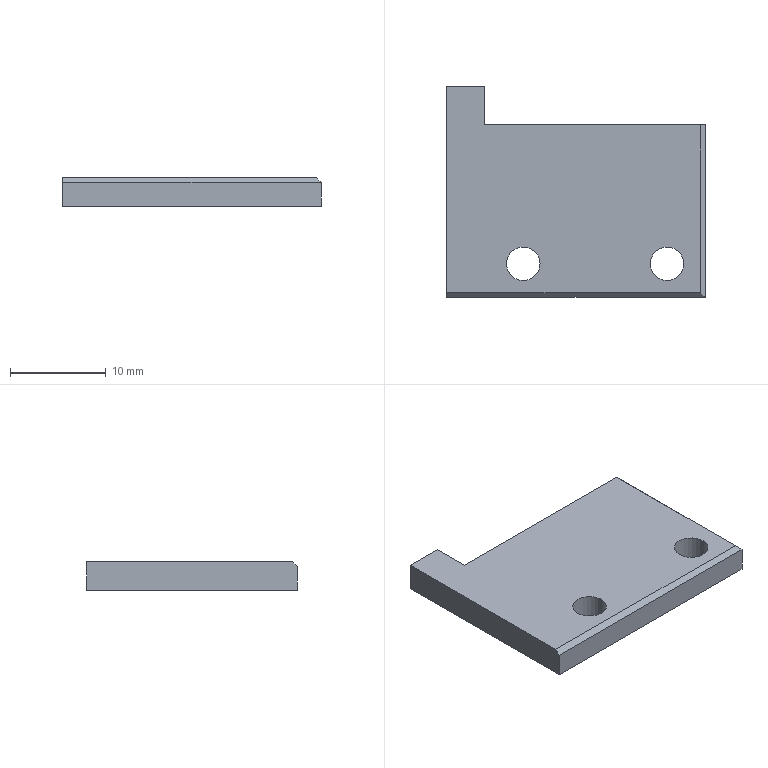Part | NX | 1 solid | 18 faces | box 27 x 22 x 3 mm | volume 1440 mm3 | plane 10 | cone 4 | cylinder 4 | commonest cylinder face diameters 3.5 x4
STEP:
#1=CARTESIAN_POINT('',(4.5,0.,1.));
#2=VERTEX_POINT('',#1);
#3=CARTESIAN_POINT('',(4.5,-22.,1.));
#4=VERTEX_POINT('',#3);
#5=CARTESIAN_POINT('',(4.5,0.,1.));
#6=DIRECTION('',(0.,-1.,0.));
#7=VECTOR('',#6,1000.);
#8=LINE('',#5,#7);
#9=EDGE_CURVE('',#2,#4,#8,.T.);
#10=ORIENTED_EDGE('',*,*,#9,.F.);
#11=CARTESIAN_POINT('',(8.5,0.,1.));
#12=VERTEX_POINT('',#11);
#13=CARTESIAN_POINT('',(0.,0.,1.));
#14=DIRECTION('',(1.,0.,0.));
#15=VECTOR('',#14,1000.);
#16=LINE('',#13,#15);
#17=EDGE_CURVE('',#2,#12,#16,.T.);
#18=ORIENTED_EDGE('',*,*,#17,.T.);
#19=CARTESIAN_POINT('',(8.5,-4.,1.));
#20=VERTEX_POINT('',#19);
#21=CARTESIAN_POINT('',(8.5,0.,1.));
#22=DIRECTION('',(0.,1.,0.));
#23=VECTOR('',#22,1000.);
#24=LINE('',#21,#23);
#25=EDGE_CURVE('',#20,#12,#24,.T.);
#26=ORIENTED_EDGE('',*,*,#25,.F.);
#27=CARTESIAN_POINT('',(31.5,-4.,1.));
#28=VERTEX_POINT('',#27);
#29=CARTESIAN_POINT('',(0.,-4.,1.));
#30=DIRECTION('',(-1.,0.,0.));
#31=VECTOR('',#30,1000.);
#32=LINE('',#29,#31);
#33=EDGE_CURVE('',#28,#20,#32,.T.);
#34=ORIENTED_EDGE('',*,*,#33,.F.);
#35=CARTESIAN_POINT('',(31.5,-22.,1.));
#36=VERTEX_POINT('',#35);
#37=CARTESIAN_POINT('',(31.5,0.,1.));
#38=DIRECTION('',(0.,1.,0.));
#39=VECTOR('',#38,1000.);
#40=LINE('',#37,#39);
#41=EDGE_CURVE('',#36,#28,#40,.T.);
#42=ORIENTED_EDGE('',*,*,#41,.F.);
#43=CARTESIAN_POINT('',(0.,-22.,1.));
#44=DIRECTION('',(1.,0.,0.));
#45=VECTOR('',#44,1000.);
#46=LINE('',#43,#45);
#47=EDGE_CURVE('',#4,#36,#46,.T.);
#48=ORIENTED_EDGE('',*,*,#47,.F.);
#49=EDGE_LOOP('',(#10,#18,#26,#34,#42,#48));
#50=FACE_BOUND('',#49,.T.);
#51=CARTESIAN_POINT('',(29.75,-18.5,1.));
#52=VERTEX_POINT('',#51);
#53=CARTESIAN_POINT('',(25.25,-18.5,1.));
#54=VERTEX_POINT('',#53);
#55=CARTESIAN_POINT('',(27.5,-18.5,1.));
#56=DIRECTION('',(0.,0.,-1.));
#57=DIRECTION('',(-1.,0.,0.));
#58=AXIS2_PLACEMENT_3D('',#55,#56,#57);
#59=CIRCLE('',#58,2.25);
#60=EDGE_CURVE('',#52,#54,#59,.T.);
#61=ORIENTED_EDGE('',*,*,#60,.F.);
#62=CARTESIAN_POINT('',(27.5,-18.5,1.));
#63=DIRECTION('',(0.,0.,-1.));
#64=DIRECTION('',(-1.,0.,0.));
#65=AXIS2_PLACEMENT_3D('',#62,#63,#64);
#66=CIRCLE('',#65,2.25);
#67=EDGE_CURVE('',#54,#52,#66,.T.);
#68=ORIENTED_EDGE('',*,*,#67,.F.);
#69=EDGE_LOOP('',(#61,#68));
#70=FACE_BOUND('',#69,.T.);
#71=CARTESIAN_POINT('',(10.25,-18.5,1.));
#72=VERTEX_POINT('',#71);
#73=CARTESIAN_POINT('',(14.75,-18.5,1.));
#74=VERTEX_POINT('',#73);
#75=CARTESIAN_POINT('',(12.5,-18.5,1.));
#76=DIRECTION('',(0.,0.,-1.));
#77=DIRECTION('',(-1.,0.,0.));
#78=AXIS2_PLACEMENT_3D('',#75,#76,#77);
#79=CIRCLE('',#78,2.25);
#80=EDGE_CURVE('',#72,#74,#79,.T.);
#81=ORIENTED_EDGE('',*,*,#80,.F.);
#82=CARTESIAN_POINT('',(12.5,-18.5,1.));
#83=DIRECTION('',(0.,0.,-1.));
#84=DIRECTION('',(-1.,0.,0.));
#85=AXIS2_PLACEMENT_3D('',#82,#83,#84);
#86=CIRCLE('',#85,2.25);
#87=EDGE_CURVE('',#74,#72,#86,.T.);
#88=ORIENTED_EDGE('',*,*,#87,.F.);
#89=EDGE_LOOP('',(#81,#88));
#90=FACE_BOUND('',#89,.T.);
#91=CARTESIAN_POINT('',(32.,0.,1.));
#92=DIRECTION('',(0.,0.,1.));
#93=DIRECTION('',(1.,0.,0.));
#94=AXIS2_PLACEMENT_3D('',#91,#92,#93);
#95=PLANE('',#94);
#96=ADVANCED_FACE('',(#50,#70,#90),#95,.F.);
#97=CARTESIAN_POINT('',(4.5,-21.5,4.));
#98=VERTEX_POINT('',#97);
#99=CARTESIAN_POINT('',(31.,-21.5,4.));
#100=VERTEX_POINT('',#99);
#101=CARTESIAN_POINT('',(0.,-21.5,4.));
#102=DIRECTION('',(1.,0.,0.));
#103=VECTOR('',#102,1000.);
#104=LINE('',#101,#103);
#105=EDGE_CURVE('',#98,#100,#104,.T.);
#106=ORIENTED_EDGE('',*,*,#105,.F.);
#107=CARTESIAN_POINT('',(4.5,-22.,3.5));
#108=VERTEX_POINT('',#107);
#109=CARTESIAN_POINT('',(4.5,-25.5,0.));
#110=DIRECTION('',(0.,-0.7071,-0.7071));
#111=VECTOR('',#110,1000.);
#112=LINE('',#109,#111);
#113=EDGE_CURVE('',#98,#108,#112,.T.);
#114=ORIENTED_EDGE('',*,*,#113,.T.);
#115=CARTESIAN_POINT('',(31.5,-22.,3.5));
#116=VERTEX_POINT('',#115);
#117=CARTESIAN_POINT('',(0.,-22.,3.5));
#118=DIRECTION('',(-1.,0.,0.));
#119=VECTOR('',#118,1000.);
#120=LINE('',#117,#119);
#121=EDGE_CURVE('',#116,#108,#120,.T.);
#122=ORIENTED_EDGE('',*,*,#121,.F.);
#123=CARTESIAN_POINT('',(35.,-25.5,0.));
#124=DIRECTION('',(0.5774,-0.5774,-0.5774));
#125=VECTOR('',#124,1000.);
#126=LINE('',#123,#125);
#127=EDGE_CURVE('',#100,#116,#126,.T.);
#128=ORIENTED_EDGE('',*,*,#127,.F.);
#129=EDGE_LOOP('',(#106,#114,#122,#128));
#130=FACE_BOUND('',#129,.T.);
#131=CARTESIAN_POINT('',(17.25,-21.75,3.75));
#132=DIRECTION('',(0.,-0.7071,0.7071));
#133=DIRECTION('',(-1.,0.,0.));
#134=AXIS2_PLACEMENT_3D('',#131,#132,#133);
#135=PLANE('',#134);
#136=ADVANCED_FACE('',(#130),#135,.T.);
#137=CARTESIAN_POINT('',(31.5,-4.,3.5));
#138=VERTEX_POINT('',#137);
#139=CARTESIAN_POINT('',(31.5,0.,3.5));
#140=DIRECTION('',(0.,1.,0.));
#141=VECTOR('',#140,1000.);
#142=LINE('',#139,#141);
#143=EDGE_CURVE('',#116,#138,#142,.T.);
#144=ORIENTED_EDGE('',*,*,#143,.F.);
#145=CARTESIAN_POINT('',(31.5,-22.,0.));
#146=DIRECTION('',(0.,0.,1.));
#147=VECTOR('',#146,1000.);
#148=LINE('',#145,#147);
#149=EDGE_CURVE('',#36,#116,#148,.T.);
#150=ORIENTED_EDGE('',*,*,#149,.F.);
#151=ORIENTED_EDGE('',*,*,#41,.T.);
#152=CARTESIAN_POINT('',(31.5,-4.,0.));
#153=DIRECTION('',(0.,0.,1.));
#154=VECTOR('',#153,1000.);
#155=LINE('',#152,#154);
#156=EDGE_CURVE('',#28,#138,#155,.T.);
#157=ORIENTED_EDGE('',*,*,#156,.T.);
#158=EDGE_LOOP('',(#144,#150,#151,#157));
#159=FACE_BOUND('',#158,.T.);
#160=CARTESIAN_POINT('',(31.5,-22.5,0.));
#161=DIRECTION('',(1.,0.,0.));
#162=DIRECTION('',(0.,1.,0.));
#163=AXIS2_PLACEMENT_3D('',#160,#161,#162);
#164=PLANE('',#163);
#165=ADVANCED_FACE('',(#159),#164,.T.);
#166=ORIENTED_EDGE('',*,*,#105,.T.);
#167=CARTESIAN_POINT('',(31.,-4.,4.));
#168=VERTEX_POINT('',#167);
#169=CARTESIAN_POINT('',(31.,0.,4.));
#170=DIRECTION('',(0.,1.,0.));
#171=VECTOR('',#170,1000.);
#172=LINE('',#169,#171);
#173=EDGE_CURVE('',#100,#168,#172,.T.);
#174=ORIENTED_EDGE('',*,*,#173,.T.);
#175=CARTESIAN_POINT('',(8.5,-4.,4.));
#176=VERTEX_POINT('',#175);
#177=CARTESIAN_POINT('',(0.,-4.,4.));
#178=DIRECTION('',(-1.,0.,0.));
#179=VECTOR('',#178,1000.);
#180=LINE('',#177,#179);
#181=EDGE_CURVE('',#168,#176,#180,.T.);
#182=ORIENTED_EDGE('',*,*,#181,.T.);
#183=CARTESIAN_POINT('',(8.5,0.,4.));
#184=VERTEX_POINT('',#183);
#185=CARTESIAN_POINT('',(8.5,0.,4.));
#186=DIRECTION('',(0.,1.,0.));
#187=VECTOR('',#186,1000.);
#188=LINE('',#185,#187);
#189=EDGE_CURVE('',#176,#184,#188,.T.);
#190=ORIENTED_EDGE('',*,*,#189,.T.);
#191=CARTESIAN_POINT('',(4.5,0.,4.));
#192=VERTEX_POINT('',#191);
#193=CARTESIAN_POINT('',(0.,0.,4.));
#194=DIRECTION('',(1.,0.,0.));
#195=VECTOR('',#194,1000.);
#196=LINE('',#193,#195);
#197=EDGE_CURVE('',#192,#184,#196,.T.);
#198=ORIENTED_EDGE('',*,*,#197,.F.);
#199=CARTESIAN_POINT('',(4.5,0.,4.));
#200=DIRECTION('',(0.,-1.,0.));
#201=VECTOR('',#200,1000.);
#202=LINE('',#199,#201);
#203=EDGE_CURVE('',#192,#98,#202,.T.);
#204=ORIENTED_EDGE('',*,*,#203,.T.);
#205=EDGE_LOOP('',(#166,#174,#182,#190,#198,#204));
#206=FACE_BOUND('',#205,.T.);
#207=CARTESIAN_POINT('',(10.75,-18.5,4.));
#208=VERTEX_POINT('',#207);
#209=CARTESIAN_POINT('',(14.25,-18.5,4.));
#210=VERTEX_POINT('',#209);
#211=CARTESIAN_POINT('',(12.5,-18.5,4.));
#212=DIRECTION('',(0.,0.,-1.));
#213=DIRECTION('',(-1.,0.,0.));
#214=AXIS2_PLACEMENT_3D('',#211,#212,#213);
#215=CIRCLE('',#214,1.75);
#216=EDGE_CURVE('',#208,#210,#215,.T.);
#217=ORIENTED_EDGE('',*,*,#216,.T.);
#218=CARTESIAN_POINT('',(12.5,-18.5,4.));
#219=DIRECTION('',(0.,0.,-1.));
#220=DIRECTION('',(-1.,0.,0.));
#221=AXIS2_PLACEMENT_3D('',#218,#219,#220);
#222=CIRCLE('',#221,1.75);
#223=EDGE_CURVE('',#210,#208,#222,.T.);
#224=ORIENTED_EDGE('',*,*,#223,.T.);
#225=EDGE_LOOP('',(#217,#224));
#226=FACE_BOUND('',#225,.T.);
#227=CARTESIAN_POINT('',(29.25,-18.5,4.));
#228=VERTEX_POINT('',#227);
#229=CARTESIAN_POINT('',(25.75,-18.5,4.));
#230=VERTEX_POINT('',#229);
#231=CARTESIAN_POINT('',(27.5,-18.5,4.));
#232=DIRECTION('',(0.,0.,-1.));
#233=DIRECTION('',(-1.,0.,0.));
#234=AXIS2_PLACEMENT_3D('',#231,#232,#233);
#235=CIRCLE('',#234,1.75);
#236=EDGE_CURVE('',#228,#230,#235,.T.);
#237=ORIENTED_EDGE('',*,*,#236,.T.);
#238=CARTESIAN_POINT('',(27.5,-18.5,4.));
#239=DIRECTION('',(0.,0.,-1.));
#240=DIRECTION('',(-1.,0.,0.));
#241=AXIS2_PLACEMENT_3D('',#238,#239,#240);
#242=CIRCLE('',#241,1.75);
#243=EDGE_CURVE('',#230,#228,#242,.T.);
#244=ORIENTED_EDGE('',*,*,#243,.T.);
#245=EDGE_LOOP('',(#237,#244));
#246=FACE_BOUND('',#245,.T.);
#247=CARTESIAN_POINT('',(0.,0.,4.));
#248=DIRECTION('',(0.,0.,1.));
#249=DIRECTION('',(1.,0.,0.));
#250=AXIS2_PLACEMENT_3D('',#247,#248,#249);
#251=PLANE('',#250);
#252=ADVANCED_FACE('',(#206,#226,#246),#251,.T.);
#253=ORIENTED_EDGE('',*,*,#203,.F.);
#254=CARTESIAN_POINT('',(4.5,0.,0.));
#255=DIRECTION('',(0.,0.,-1.));
#256=VECTOR('',#255,1000.);
#257=LINE('',#254,#256);
#258=EDGE_CURVE('',#192,#2,#257,.T.);
#259=ORIENTED_EDGE('',*,*,#258,.T.);
#260=ORIENTED_EDGE('',*,*,#9,.T.);
#261=CARTESIAN_POINT('',(4.5,-22.,0.));
#262=DIRECTION('',(0.,0.,-1.));
#263=VECTOR('',#262,1000.);
#264=LINE('',#261,#263);
#265=EDGE_CURVE('',#108,#4,#264,.T.);
#266=ORIENTED_EDGE('',*,*,#265,.F.);
#267=ORIENTED_EDGE('',*,*,#113,.F.);
#268=EDGE_LOOP('',(#253,#259,#260,#266,#267));
#269=FACE_BOUND('',#268,.T.);
#270=CARTESIAN_POINT('',(4.5,-8.5,-11.));
#271=DIRECTION('',(1.,0.,0.));
#272=DIRECTION('',(0.,1.,0.));
#273=AXIS2_PLACEMENT_3D('',#270,#271,#272);
#274=PLANE('',#273);
#275=ADVANCED_FACE('',(#269),#274,.F.);
#276=ORIENTED_EDGE('',*,*,#197,.T.);
#277=CARTESIAN_POINT('',(8.5,0.,0.));
#278=DIRECTION('',(0.,0.,-1.));
#279=VECTOR('',#278,1000.);
#280=LINE('',#277,#279);
#281=EDGE_CURVE('',#184,#12,#280,.T.);
#282=ORIENTED_EDGE('',*,*,#281,.T.);
#283=ORIENTED_EDGE('',*,*,#17,.F.);
#284=ORIENTED_EDGE('',*,*,#258,.F.);
#285=EDGE_LOOP('',(#276,#282,#283,#284));
#286=FACE_BOUND('',#285,.T.);
#287=CARTESIAN_POINT('',(32.,0.,0.));
#288=DIRECTION('',(0.,1.,0.));
#289=DIRECTION('',(1.,0.,0.));
#290=AXIS2_PLACEMENT_3D('',#287,#288,#289);
#291=PLANE('',#290);
#292=ADVANCED_FACE('',(#286),#291,.T.);
#293=ORIENTED_EDGE('',*,*,#25,.T.);
#294=ORIENTED_EDGE('',*,*,#281,.F.);
#295=ORIENTED_EDGE('',*,*,#189,.F.);
#296=CARTESIAN_POINT('',(8.5,-4.,0.));
#297=DIRECTION('',(0.,0.,1.));
#298=VECTOR('',#297,1000.);
#299=LINE('',#296,#298);
#300=EDGE_CURVE('',#20,#176,#299,.T.);
#301=ORIENTED_EDGE('',*,*,#300,.F.);
#302=EDGE_LOOP('',(#293,#294,#295,#301));
#303=FACE_BOUND('',#302,.T.);
#304=CARTESIAN_POINT('',(8.5,0.,5.));
#305=DIRECTION('',(-1.,0.,0.));
#306=DIRECTION('',(0.,0.,1.));
#307=AXIS2_PLACEMENT_3D('',#304,#305,#306);
#308=PLANE('',#307);
#309=ADVANCED_FACE('',(#303),#308,.F.);
#310=ORIENTED_EDGE('',*,*,#33,.T.);
#311=ORIENTED_EDGE('',*,*,#300,.T.);
#312=ORIENTED_EDGE('',*,*,#181,.F.);
#313=CARTESIAN_POINT('',(35.,-4.,0.));
#314=DIRECTION('',(-0.7071,0.,0.7071));
#315=VECTOR('',#314,1000.);
#316=LINE('',#313,#315);
#317=EDGE_CURVE('',#138,#168,#316,.T.);
#318=ORIENTED_EDGE('',*,*,#317,.F.);
#319=ORIENTED_EDGE('',*,*,#156,.F.);
#320=EDGE_LOOP('',(#310,#311,#312,#318,#319));
#321=FACE_BOUND('',#320,.T.);
#322=CARTESIAN_POINT('',(3.,-4.,5.));
#323=DIRECTION('',(0.,-1.,0.));
#324=DIRECTION('',(0.,0.,-1.));
#325=AXIS2_PLACEMENT_3D('',#322,#323,#324);
#326=PLANE('',#325);
#327=ADVANCED_FACE('',(#321),#326,.F.);
#328=ORIENTED_EDGE('',*,*,#60,.T.);
#329=CARTESIAN_POINT('',(25.75,-18.5,1.5));
#330=VERTEX_POINT('',#329);
#331=CARTESIAN_POINT('',(25.25,-18.5,1.));
#332=DIRECTION('',(-0.7071,0.,-0.7071));
#333=VECTOR('',#332,1000.);
#334=LINE('',#331,#333);
#335=EDGE_CURVE('',#54,#330,#334,.F.);
#336=ORIENTED_EDGE('',*,*,#335,.T.);
#337=CARTESIAN_POINT('',(29.25,-18.5,1.5));
#338=VERTEX_POINT('',#337);
#339=CARTESIAN_POINT('',(27.5,-18.5,1.5));
#340=DIRECTION('',(0.,0.,-1.));
#341=DIRECTION('',(-1.,0.,0.));
#342=AXIS2_PLACEMENT_3D('',#339,#340,#341);
#343=CIRCLE('',#342,1.75);
#344=EDGE_CURVE('',#338,#330,#343,.T.);
#345=ORIENTED_EDGE('',*,*,#344,.F.);
#346=CARTESIAN_POINT('',(29.75,-18.5,1.));
#347=DIRECTION('',(0.7071,0.,-0.7071));
#348=VECTOR('',#347,1000.);
#349=LINE('',#346,#348);
#350=EDGE_CURVE('',#52,#338,#349,.F.);
#351=ORIENTED_EDGE('',*,*,#350,.F.);
#352=EDGE_LOOP('',(#328,#336,#345,#351));
#353=FACE_BOUND('',#352,.T.);
#354=CARTESIAN_POINT('',(27.5,-18.5,1.));
#355=DIRECTION('',(0.,0.,-1.));
#356=DIRECTION('',(-1.,0.,0.));
#357=AXIS2_PLACEMENT_3D('',#354,#355,#356);
#358=CONICAL_SURFACE('',#357,2.25,0.7854);
#359=ADVANCED_FACE('',(#353),#358,.F.);
#360=ORIENTED_EDGE('',*,*,#149,.T.);
#361=ORIENTED_EDGE('',*,*,#121,.T.);
#362=ORIENTED_EDGE('',*,*,#265,.T.);
#363=ORIENTED_EDGE('',*,*,#47,.T.);
#364=EDGE_LOOP('',(#360,#361,#362,#363));
#365=FACE_BOUND('',#364,.T.);
#366=CARTESIAN_POINT('',(0.,-22.,0.));
#367=DIRECTION('',(0.,-1.,0.));
#368=DIRECTION('',(0.,0.,-1.));
#369=AXIS2_PLACEMENT_3D('',#366,#367,#368);
#370=PLANE('',#369);
#371=ADVANCED_FACE('',(#365),#370,.T.);
#372=ORIENTED_EDGE('',*,*,#80,.T.);
#373=CARTESIAN_POINT('',(14.25,-18.5,1.5));
#374=VERTEX_POINT('',#373);
#375=CARTESIAN_POINT('',(14.75,-18.5,1.));
#376=DIRECTION('',(0.7071,0.,-0.7071));
#377=VECTOR('',#376,1000.);
#378=LINE('',#375,#377);
#379=EDGE_CURVE('',#374,#74,#378,.T.);
#380=ORIENTED_EDGE('',*,*,#379,.F.);
#381=CARTESIAN_POINT('',(10.75,-18.5,1.5));
#382=VERTEX_POINT('',#381);
#383=CARTESIAN_POINT('',(12.5,-18.5,1.5));
#384=DIRECTION('',(0.,0.,-1.));
#385=DIRECTION('',(-1.,0.,0.));
#386=AXIS2_PLACEMENT_3D('',#383,#384,#385);
#387=CIRCLE('',#386,1.75);
#388=EDGE_CURVE('',#382,#374,#387,.T.);
#389=ORIENTED_EDGE('',*,*,#388,.F.);
#390=CARTESIAN_POINT('',(10.25,-18.5,1.));
#391=DIRECTION('',(-0.7071,0.,-0.7071));
#392=VECTOR('',#391,1000.);
#393=LINE('',#390,#392);
#394=EDGE_CURVE('',#382,#72,#393,.T.);
#395=ORIENTED_EDGE('',*,*,#394,.T.);
#396=EDGE_LOOP('',(#372,#380,#389,#395));
#397=FACE_BOUND('',#396,.T.);
#398=CARTESIAN_POINT('',(12.5,-18.5,1.));
#399=DIRECTION('',(0.,0.,-1.));
#400=DIRECTION('',(-1.,0.,0.));
#401=AXIS2_PLACEMENT_3D('',#398,#399,#400);
#402=CONICAL_SURFACE('',#401,2.25,0.7854);
#403=ADVANCED_FACE('',(#397),#402,.F.);
#404=CARTESIAN_POINT('',(27.5,-18.5,1.5));
#405=DIRECTION('',(0.,0.,-1.));
#406=DIRECTION('',(-1.,0.,0.));
#407=AXIS2_PLACEMENT_3D('',#404,#405,#406);
#408=CIRCLE('',#407,1.75);
#409=EDGE_CURVE('',#330,#338,#408,.T.);
#410=ORIENTED_EDGE('',*,*,#409,.T.);
#411=CARTESIAN_POINT('',(29.25,-18.5,5.));
#412=DIRECTION('',(0.,0.,-1.));
#413=VECTOR('',#412,1000.);
#414=LINE('',#411,#413);
#415=EDGE_CURVE('',#228,#338,#414,.T.);
#416=ORIENTED_EDGE('',*,*,#415,.F.);
#417=ORIENTED_EDGE('',*,*,#243,.F.);
#418=CARTESIAN_POINT('',(25.75,-18.5,5.));
#419=DIRECTION('',(0.,0.,-1.));
#420=VECTOR('',#419,1000.);
#421=LINE('',#418,#420);
#422=EDGE_CURVE('',#230,#330,#421,.T.);
#423=ORIENTED_EDGE('',*,*,#422,.T.);
#424=EDGE_LOOP('',(#410,#416,#417,#423));
#425=FACE_BOUND('',#424,.T.);
#426=CARTESIAN_POINT('',(27.5,-18.5,5.));
#427=DIRECTION('',(0.,0.,-1.));
#428=DIRECTION('',(-1.,0.,0.));
#429=AXIS2_PLACEMENT_3D('',#426,#427,#428);
#430=CYLINDRICAL_SURFACE('',#429,1.75);
#431=ADVANCED_FACE('',(#425),#430,.F.);
#432=CARTESIAN_POINT('',(12.5,-18.5,1.5));
#433=DIRECTION('',(0.,0.,-1.));
#434=DIRECTION('',(-1.,0.,0.));
#435=AXIS2_PLACEMENT_3D('',#432,#433,#434);
#436=CIRCLE('',#435,1.75);
#437=EDGE_CURVE('',#374,#382,#436,.T.);
#438=ORIENTED_EDGE('',*,*,#437,.T.);
#439=CARTESIAN_POINT('',(10.75,-18.5,5.));
#440=DIRECTION('',(0.,0.,-1.));
#441=VECTOR('',#440,1000.);
#442=LINE('',#439,#441);
#443=EDGE_CURVE('',#382,#208,#442,.F.);
#444=ORIENTED_EDGE('',*,*,#443,.T.);
#445=ORIENTED_EDGE('',*,*,#223,.F.);
#446=CARTESIAN_POINT('',(14.25,-18.5,5.));
#447=DIRECTION('',(0.,0.,-1.));
#448=VECTOR('',#447,1000.);
#449=LINE('',#446,#448);
#450=EDGE_CURVE('',#374,#210,#449,.F.);
#451=ORIENTED_EDGE('',*,*,#450,.F.);
#452=EDGE_LOOP('',(#438,#444,#445,#451));
#453=FACE_BOUND('',#452,.T.);
#454=CARTESIAN_POINT('',(12.5,-18.5,5.));
#455=DIRECTION('',(0.,0.,-1.));
#456=DIRECTION('',(-1.,0.,0.));
#457=AXIS2_PLACEMENT_3D('',#454,#455,#456);
#458=CYLINDRICAL_SURFACE('',#457,1.75);
#459=ADVANCED_FACE('',(#453),#458,.F.);
#460=ORIENTED_EDGE('',*,*,#127,.T.);
#461=ORIENTED_EDGE('',*,*,#143,.T.);
#462=ORIENTED_EDGE('',*,*,#317,.T.);
#463=ORIENTED_EDGE('',*,*,#173,.F.);
#464=EDGE_LOOP('',(#460,#461,#462,#463));
#465=FACE_BOUND('',#464,.T.);
#466=CARTESIAN_POINT('',(31.25,-13.25,3.75));
#467=DIRECTION('',(0.7071,0.,0.7071));
#468=DIRECTION('',(0.,-1.,0.));
#469=AXIS2_PLACEMENT_3D('',#466,#467,#468);
#470=PLANE('',#469);
#471=ADVANCED_FACE('',(#465),#470,.T.);
#472=ORIENTED_EDGE('',*,*,#437,.F.);
#473=ORIENTED_EDGE('',*,*,#379,.T.);
#474=ORIENTED_EDGE('',*,*,#87,.T.);
#475=ORIENTED_EDGE('',*,*,#394,.F.);
#476=EDGE_LOOP('',(#472,#473,#474,#475));
#477=FACE_BOUND('',#476,.T.);
#478=CARTESIAN_POINT('',(12.5,-18.5,1.));
#479=DIRECTION('',(0.,0.,-1.));
#480=DIRECTION('',(-1.,0.,0.));
#481=AXIS2_PLACEMENT_3D('',#478,#479,#480);
#482=CONICAL_SURFACE('',#481,2.25,0.7854);
#483=ADVANCED_FACE('',(#477),#482,.F.);
#484=ORIENTED_EDGE('',*,*,#216,.F.);
#485=ORIENTED_EDGE('',*,*,#443,.F.);
#486=ORIENTED_EDGE('',*,*,#388,.T.);
#487=ORIENTED_EDGE('',*,*,#450,.T.);
#488=EDGE_LOOP('',(#484,#485,#486,#487));
#489=FACE_BOUND('',#488,.T.);
#490=CARTESIAN_POINT('',(12.5,-18.5,5.));
#491=DIRECTION('',(0.,0.,-1.));
#492=DIRECTION('',(-1.,0.,0.));
#493=AXIS2_PLACEMENT_3D('',#490,#491,#492);
#494=CYLINDRICAL_SURFACE('',#493,1.75);
#495=ADVANCED_FACE('',(#489),#494,.F.);
#496=ORIENTED_EDGE('',*,*,#409,.F.);
#497=ORIENTED_EDGE('',*,*,#335,.F.);
#498=ORIENTED_EDGE('',*,*,#67,.T.);
#499=ORIENTED_EDGE('',*,*,#350,.T.);
#500=EDGE_LOOP('',(#496,#497,#498,#499));
#501=FACE_BOUND('',#500,.T.);
#502=CARTESIAN_POINT('',(27.5,-18.5,1.));
#503=DIRECTION('',(0.,0.,-1.));
#504=DIRECTION('',(-1.,0.,0.));
#505=AXIS2_PLACEMENT_3D('',#502,#503,#504);
#506=CONICAL_SURFACE('',#505,2.25,0.7854);
#507=ADVANCED_FACE('',(#501),#506,.F.);
#508=ORIENTED_EDGE('',*,*,#236,.F.);
#509=ORIENTED_EDGE('',*,*,#415,.T.);
#510=ORIENTED_EDGE('',*,*,#344,.T.);
#511=ORIENTED_EDGE('',*,*,#422,.F.);
#512=EDGE_LOOP('',(#508,#509,#510,#511));
#513=FACE_BOUND('',#512,.T.);
#514=CARTESIAN_POINT('',(27.5,-18.5,5.));
#515=DIRECTION('',(0.,0.,-1.));
#516=DIRECTION('',(-1.,0.,0.));
#517=AXIS2_PLACEMENT_3D('',#514,#515,#516);
#518=CYLINDRICAL_SURFACE('',#517,1.75);
#519=ADVANCED_FACE('',(#513),#518,.F.);
#520=CLOSED_SHELL('',(#96,#136,#165,#252,#275,#292,#309,#327,#359,#371,#403,#431,#459,#471,#483,#495,#507,#519));
#521=MANIFOLD_SOLID_BREP('',#520);
#522=(LENGTH_UNIT()NAMED_UNIT(*)SI_UNIT(.MILLI.,.METRE.));
#523=UNCERTAINTY_MEASURE_WITH_UNIT(LENGTH_MEASURE(0.00001),#522,'','');
#524=(NAMED_UNIT(*)PLANE_ANGLE_UNIT()SI_UNIT($,.RADIAN.));
#525=(NAMED_UNIT(*)SI_UNIT($,.STERADIAN.)SOLID_ANGLE_UNIT());
#526=(GEOMETRIC_REPRESENTATION_CONTEXT(3)GLOBAL_UNCERTAINTY_ASSIGNED_CONTEXT((#523))GLOBAL_UNIT_ASSIGNED_CONTEXT((#522,#524,#525))REPRESENTATION_CONTEXT('',''));
#527=ADVANCED_BREP_SHAPE_REPRESENTATION('',(#521),#526);